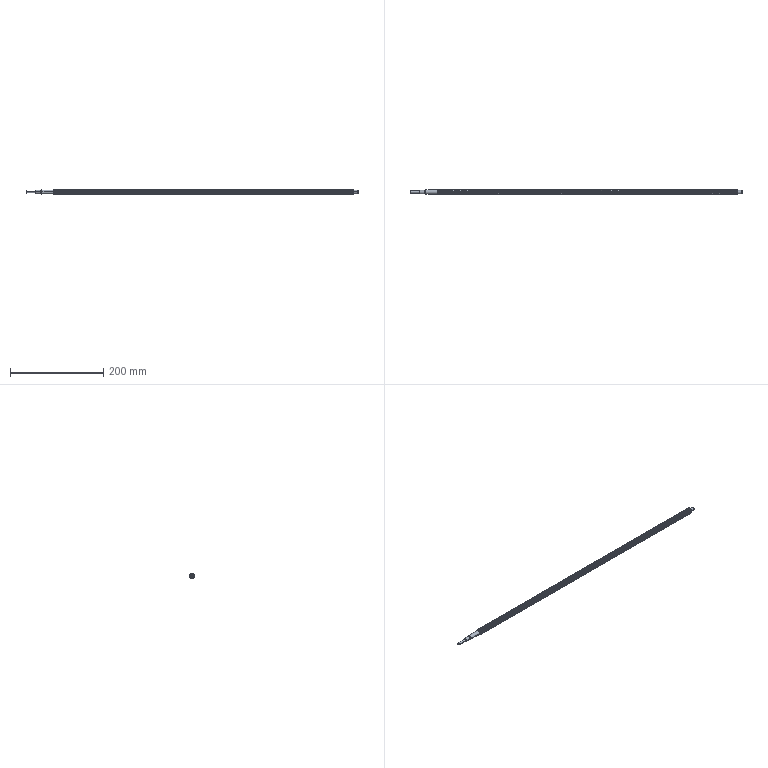Part | Creo | features DATUM PLANE 3, COORDINATE SYSTEM 1, CURVE 1, CUT 1, PROTRUSION 1 | 1 solid | 509 faces | box 712.5 x 12 x 12.001 mm | volume 63984 mm3 | cylinder 438 | spline 54 | cone 10 | plane 7 | commonest cylinder face diameters 12 x428 7 x4 5 x2 6 x2 9 x2